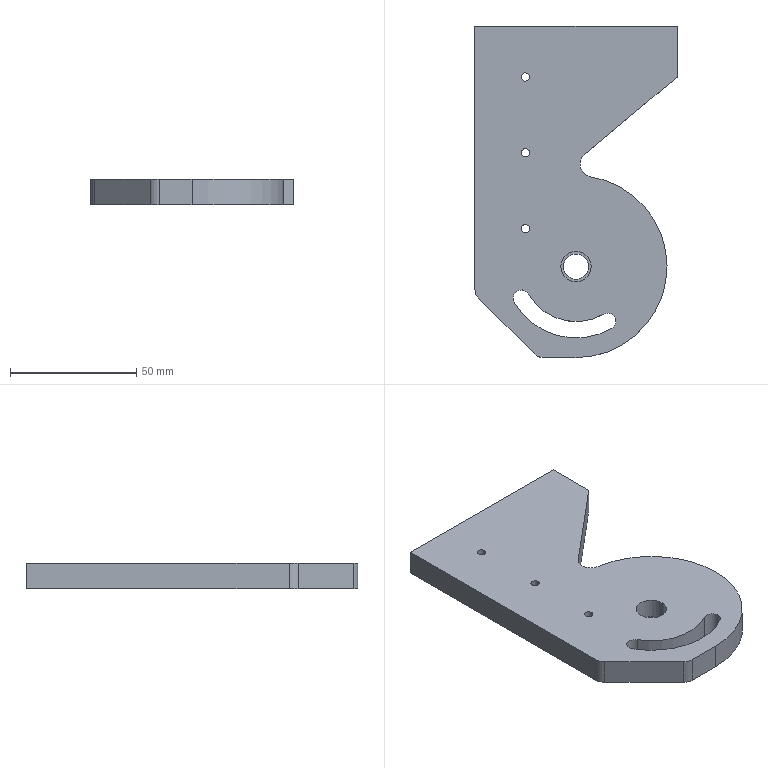Part | SolidWorks | features HoleWzd 3, Cut 1, Extrusion 1, Fillet 1, ICE 1 | 1 solid | 37 faces | box 80 x 131 x 10 mm | volume 79591 mm3 | cylinder 24 | plane 9 | cone 4 | commonest cylinder face diameters 3.3 x6 10 x6 5 x4 6.5 x3 12 x2 43.5 x1
STEP:
#1=CARTESIAN_POINT('',(-18.35,35.,5.));
#2=VERTEX_POINT('',#1);
#3=CARTESIAN_POINT('',(-21.65,35.,5.));
#4=VERTEX_POINT('',#3);
#5=CARTESIAN_POINT('',(-20.,35.,5.));
#6=DIRECTION('',(0.,0.,-1.));
#7=DIRECTION('',(-1.,0.,0.));
#8=AXIS2_PLACEMENT_3D('',#5,#6,#7);
#9=CIRCLE('',#8,1.65);
#10=EDGE_CURVE('',#2,#4,#9,.T.);
#11=ORIENTED_EDGE('',*,*,#10,.F.);
#12=CARTESIAN_POINT('',(-18.35,35.,-5.));
#13=VERTEX_POINT('',#12);
#14=CARTESIAN_POINT('',(-18.35,35.,-5.));
#15=DIRECTION('',(0.,0.,-1.));
#16=VECTOR('',#15,1000.);
#17=LINE('',#14,#16);
#18=EDGE_CURVE('',#2,#13,#17,.T.);
#19=ORIENTED_EDGE('',*,*,#18,.T.);
#20=CARTESIAN_POINT('',(-21.65,35.,-5.));
#21=VERTEX_POINT('',#20);
#22=CARTESIAN_POINT('',(-20.,35.,-5.));
#23=DIRECTION('',(0.,0.,-1.));
#24=DIRECTION('',(-1.,0.,0.));
#25=AXIS2_PLACEMENT_3D('',#22,#23,#24);
#26=CIRCLE('',#25,1.65);
#27=EDGE_CURVE('',#13,#21,#26,.T.);
#28=ORIENTED_EDGE('',*,*,#27,.T.);
#29=CARTESIAN_POINT('',(-21.65,35.,-5.));
#30=DIRECTION('',(0.,0.,-1.));
#31=VECTOR('',#30,1000.);
#32=LINE('',#29,#31);
#33=EDGE_CURVE('',#4,#21,#32,.T.);
#34=ORIENTED_EDGE('',*,*,#33,.F.);
#35=EDGE_LOOP('',(#11,#19,#28,#34));
#36=FACE_OUTER_BOUND('',#35,.T.);
#37=CARTESIAN_POINT('',(-20.,35.,-5.));
#38=DIRECTION('',(0.,0.,-1.));
#39=DIRECTION('',(-1.,0.,0.));
#40=AXIS2_PLACEMENT_3D('',#37,#38,#39);
#41=CYLINDRICAL_SURFACE('',#40,1.65);
#42=ADVANCED_FACE('',(#36),#41,.F.);
#43=CARTESIAN_POINT('',(-18.35,65.,5.));
#44=VERTEX_POINT('',#43);
#45=CARTESIAN_POINT('',(-21.65,65.,5.));
#46=VERTEX_POINT('',#45);
#47=CARTESIAN_POINT('',(-20.,65.,5.));
#48=DIRECTION('',(0.,0.,-1.));
#49=DIRECTION('',(-1.,0.,0.));
#50=AXIS2_PLACEMENT_3D('',#47,#48,#49);
#51=CIRCLE('',#50,1.65);
#52=EDGE_CURVE('',#44,#46,#51,.T.);
#53=ORIENTED_EDGE('',*,*,#52,.F.);
#54=CARTESIAN_POINT('',(-18.35,65.,-5.));
#55=VERTEX_POINT('',#54);
#56=CARTESIAN_POINT('',(-18.35,65.,-5.));
#57=DIRECTION('',(0.,0.,-1.));
#58=VECTOR('',#57,1000.);
#59=LINE('',#56,#58);
#60=EDGE_CURVE('',#44,#55,#59,.T.);
#61=ORIENTED_EDGE('',*,*,#60,.T.);
#62=CARTESIAN_POINT('',(-21.65,65.,-5.));
#63=VERTEX_POINT('',#62);
#64=CARTESIAN_POINT('',(-20.,65.,-5.));
#65=DIRECTION('',(0.,0.,-1.));
#66=DIRECTION('',(-1.,0.,0.));
#67=AXIS2_PLACEMENT_3D('',#64,#65,#66);
#68=CIRCLE('',#67,1.65);
#69=EDGE_CURVE('',#55,#63,#68,.T.);
#70=ORIENTED_EDGE('',*,*,#69,.T.);
#71=CARTESIAN_POINT('',(-21.65,65.,-5.));
#72=DIRECTION('',(0.,0.,-1.));
#73=VECTOR('',#72,1000.);
#74=LINE('',#71,#73);
#75=EDGE_CURVE('',#46,#63,#74,.T.);
#76=ORIENTED_EDGE('',*,*,#75,.F.);
#77=EDGE_LOOP('',(#53,#61,#70,#76));
#78=FACE_OUTER_BOUND('',#77,.T.);
#79=CARTESIAN_POINT('',(-20.,65.,-5.));
#80=DIRECTION('',(0.,0.,-1.));
#81=DIRECTION('',(-1.,0.,0.));
#82=AXIS2_PLACEMENT_3D('',#79,#80,#81);
#83=CYLINDRICAL_SURFACE('',#82,1.65);
#84=ADVANCED_FACE('',(#78),#83,.F.);
#85=CARTESIAN_POINT('',(-18.35,5.,5.));
#86=VERTEX_POINT('',#85);
#87=CARTESIAN_POINT('',(-21.65,5.,5.));
#88=VERTEX_POINT('',#87);
#89=CARTESIAN_POINT('',(-20.,5.,5.));
#90=DIRECTION('',(0.,0.,-1.));
#91=DIRECTION('',(-1.,0.,0.));
#92=AXIS2_PLACEMENT_3D('',#89,#90,#91);
#93=CIRCLE('',#92,1.65);
#94=EDGE_CURVE('',#86,#88,#93,.T.);
#95=ORIENTED_EDGE('',*,*,#94,.F.);
#96=CARTESIAN_POINT('',(-18.35,5.,-5.));
#97=VERTEX_POINT('',#96);
#98=CARTESIAN_POINT('',(-18.35,5.,-5.));
#99=DIRECTION('',(0.,0.,-1.));
#100=VECTOR('',#99,1000.);
#101=LINE('',#98,#100);
#102=EDGE_CURVE('',#86,#97,#101,.T.);
#103=ORIENTED_EDGE('',*,*,#102,.T.);
#104=CARTESIAN_POINT('',(-21.65,5.,-5.));
#105=VERTEX_POINT('',#104);
#106=CARTESIAN_POINT('',(-20.,5.,-5.));
#107=DIRECTION('',(0.,0.,-1.));
#108=DIRECTION('',(-1.,0.,0.));
#109=AXIS2_PLACEMENT_3D('',#106,#107,#108);
#110=CIRCLE('',#109,1.65);
#111=EDGE_CURVE('',#97,#105,#110,.T.);
#112=ORIENTED_EDGE('',*,*,#111,.T.);
#113=CARTESIAN_POINT('',(-21.65,5.,-5.));
#114=DIRECTION('',(0.,0.,-1.));
#115=VECTOR('',#114,1000.);
#116=LINE('',#113,#115);
#117=EDGE_CURVE('',#88,#105,#116,.T.);
#118=ORIENTED_EDGE('',*,*,#117,.F.);
#119=EDGE_LOOP('',(#95,#103,#112,#118));
#120=FACE_OUTER_BOUND('',#119,.T.);
#121=CARTESIAN_POINT('',(-20.,5.,-5.));
#122=DIRECTION('',(0.,0.,-1.));
#123=DIRECTION('',(-1.,0.,0.));
#124=AXIS2_PLACEMENT_3D('',#121,#122,#123);
#125=CYLINDRICAL_SURFACE('',#124,1.65);
#126=ADVANCED_FACE('',(#120),#125,.F.);
#127=CARTESIAN_POINT('',(-28.,68.,-2.5));
#128=VERTEX_POINT('',#127);
#129=CARTESIAN_POINT('',(-28.,68.,2.5));
#130=VERTEX_POINT('',#129);
#131=CARTESIAN_POINT('',(-28.,68.,0.));
#132=DIRECTION('',(0.,1.,0.));
#133=DIRECTION('',(0.,0.,1.));
#134=AXIS2_PLACEMENT_3D('',#131,#132,#133);
#135=CIRCLE('',#134,2.5);
#136=EDGE_CURVE('',#128,#130,#135,.T.);
#137=ORIENTED_EDGE('',*,*,#136,.F.);
#138=CARTESIAN_POINT('',(-28.,85.,-2.5));
#139=VERTEX_POINT('',#138);
#140=CARTESIAN_POINT('',(-28.,85.,-2.5));
#141=DIRECTION('',(0.,1.,0.));
#142=VECTOR('',#141,1000.);
#143=LINE('',#140,#142);
#144=EDGE_CURVE('',#128,#139,#143,.T.);
#145=ORIENTED_EDGE('',*,*,#144,.T.);
#146=CARTESIAN_POINT('',(-28.,85.,2.5));
#147=VERTEX_POINT('',#146);
#148=CARTESIAN_POINT('',(-28.,85.,0.));
#149=DIRECTION('',(0.,1.,0.));
#150=DIRECTION('',(0.,0.,1.));
#151=AXIS2_PLACEMENT_3D('',#148,#149,#150);
#152=CIRCLE('',#151,2.5);
#153=EDGE_CURVE('',#139,#147,#152,.T.);
#154=ORIENTED_EDGE('',*,*,#153,.T.);
#155=CARTESIAN_POINT('',(-28.,85.,2.5));
#156=DIRECTION('',(0.,1.,0.));
#157=VECTOR('',#156,1000.);
#158=LINE('',#155,#157);
#159=EDGE_CURVE('',#130,#147,#158,.T.);
#160=ORIENTED_EDGE('',*,*,#159,.F.);
#161=EDGE_LOOP('',(#137,#145,#154,#160));
#162=FACE_OUTER_BOUND('',#161,.T.);
#163=CARTESIAN_POINT('',(-28.,85.,0.));
#164=DIRECTION('',(0.,1.,0.));
#165=DIRECTION('',(0.,0.,1.));
#166=AXIS2_PLACEMENT_3D('',#163,#164,#165);
#167=CYLINDRICAL_SURFACE('',#166,2.5);
#168=ADVANCED_FACE('',(#162),#167,.F.);
#169=CARTESIAN_POINT('',(-28.,66.498,0.));
#170=VERTEX_POINT('',#169);
#171=CARTESIAN_POINT('',(-28.,68.,2.5));
#172=DIRECTION('',(0.,0.515,0.8572));
#173=VECTOR('',#172,1000.);
#174=LINE('',#171,#173);
#175=EDGE_CURVE('',#170,#130,#174,.T.);
#176=ORIENTED_EDGE('',*,*,#175,.F.);
#177=CARTESIAN_POINT('',(-28.,68.,-2.5));
#178=DIRECTION('',(0.,0.515,-0.8572));
#179=VECTOR('',#178,1000.);
#180=LINE('',#177,#179);
#181=EDGE_CURVE('',#170,#128,#180,.T.);
#182=ORIENTED_EDGE('',*,*,#181,.T.);
#183=ORIENTED_EDGE('',*,*,#136,.T.);
#184=EDGE_LOOP('',(#176,#182,#183));
#185=FACE_OUTER_BOUND('',#184,.T.);
#186=CARTESIAN_POINT('',(-28.,68.,0.));
#187=DIRECTION('',(0.,1.,0.));
#188=DIRECTION('',(0.,0.,1.));
#189=AXIS2_PLACEMENT_3D('',#186,#187,#188);
#190=CONICAL_SURFACE('',#189,2.5,1.03);
#191=ADVANCED_FACE('',(#185),#190,.F.);
#192=CARTESIAN_POINT('',(28.,68.,-2.5));
#193=VERTEX_POINT('',#192);
#194=CARTESIAN_POINT('',(28.,68.,2.5));
#195=VERTEX_POINT('',#194);
#196=CARTESIAN_POINT('',(28.,68.,0.));
#197=DIRECTION('',(0.,1.,0.));
#198=DIRECTION('',(0.,0.,1.));
#199=AXIS2_PLACEMENT_3D('',#196,#197,#198);
#200=CIRCLE('',#199,2.5);
#201=EDGE_CURVE('',#193,#195,#200,.T.);
#202=ORIENTED_EDGE('',*,*,#201,.F.);
#203=CARTESIAN_POINT('',(28.,85.,-2.5));
#204=VERTEX_POINT('',#203);
#205=CARTESIAN_POINT('',(28.,85.,-2.5));
#206=DIRECTION('',(0.,1.,0.));
#207=VECTOR('',#206,1000.);
#208=LINE('',#205,#207);
#209=EDGE_CURVE('',#193,#204,#208,.T.);
#210=ORIENTED_EDGE('',*,*,#209,.T.);
#211=CARTESIAN_POINT('',(28.,85.,2.5));
#212=VERTEX_POINT('',#211);
#213=CARTESIAN_POINT('',(28.,85.,0.));
#214=DIRECTION('',(0.,1.,0.));
#215=DIRECTION('',(0.,0.,1.));
#216=AXIS2_PLACEMENT_3D('',#213,#214,#215);
#217=CIRCLE('',#216,2.5);
#218=EDGE_CURVE('',#204,#212,#217,.T.);
#219=ORIENTED_EDGE('',*,*,#218,.T.);
#220=CARTESIAN_POINT('',(28.,85.,2.5));
#221=DIRECTION('',(0.,1.,0.));
#222=VECTOR('',#221,1000.);
#223=LINE('',#220,#222);
#224=EDGE_CURVE('',#195,#212,#223,.T.);
#225=ORIENTED_EDGE('',*,*,#224,.F.);
#226=EDGE_LOOP('',(#202,#210,#219,#225));
#227=FACE_OUTER_BOUND('',#226,.T.);
#228=CARTESIAN_POINT('',(28.,85.,0.));
#229=DIRECTION('',(0.,1.,0.));
#230=DIRECTION('',(0.,0.,1.));
#231=AXIS2_PLACEMENT_3D('',#228,#229,#230);
#232=CYLINDRICAL_SURFACE('',#231,2.5);
#233=ADVANCED_FACE('',(#227),#232,.F.);
#234=CARTESIAN_POINT('',(28.,66.498,0.));
#235=VERTEX_POINT('',#234);
#236=CARTESIAN_POINT('',(28.,68.,2.5));
#237=DIRECTION('',(0.,0.515,0.8572));
#238=VECTOR('',#237,1000.);
#239=LINE('',#236,#238);
#240=EDGE_CURVE('',#235,#195,#239,.T.);
#241=ORIENTED_EDGE('',*,*,#240,.F.);
#242=CARTESIAN_POINT('',(28.,68.,-2.5));
#243=DIRECTION('',(0.,0.515,-0.8572));
#244=VECTOR('',#243,1000.);
#245=LINE('',#242,#244);
#246=EDGE_CURVE('',#235,#193,#245,.T.);
#247=ORIENTED_EDGE('',*,*,#246,.T.);
#248=ORIENTED_EDGE('',*,*,#201,.T.);
#249=EDGE_LOOP('',(#241,#247,#248));
#250=FACE_OUTER_BOUND('',#249,.T.);
#251=CARTESIAN_POINT('',(28.,68.,0.));
#252=DIRECTION('',(0.,1.,0.));
#253=DIRECTION('',(0.,0.,1.));
#254=AXIS2_PLACEMENT_3D('',#251,#252,#253);
#255=CONICAL_SURFACE('',#254,2.5,1.03);
#256=ADVANCED_FACE('',(#250),#255,.F.);
#257=CARTESIAN_POINT('',(1.618,30.462,5.));
#258=VERTEX_POINT('',#257);
#259=CARTESIAN_POINT('',(3.404,34.293,5.));
#260=VERTEX_POINT('',#259);
#261=CARTESIAN_POINT('',(6.618,30.462,5.));
#262=DIRECTION('',(0.,0.,-1.));
#263=DIRECTION('',(-1.,0.,0.));
#264=AXIS2_PLACEMENT_3D('',#261,#262,#263);
#265=CIRCLE('',#264,5.);
#266=EDGE_CURVE('',#258,#260,#265,.T.);
#267=ORIENTED_EDGE('',*,*,#266,.F.);
#268=CARTESIAN_POINT('',(1.618,30.462,-5.));
#269=VERTEX_POINT('',#268);
#270=CARTESIAN_POINT('',(1.618,30.462,5.));
#271=DIRECTION('',(0.,0.,-1.));
#272=VECTOR('',#271,1000.);
#273=LINE('',#270,#272);
#274=EDGE_CURVE('',#258,#269,#273,.T.);
#275=ORIENTED_EDGE('',*,*,#274,.T.);
#276=CARTESIAN_POINT('',(3.404,34.293,-5.));
#277=VERTEX_POINT('',#276);
#278=CARTESIAN_POINT('',(6.618,30.462,-5.));
#279=DIRECTION('',(0.,0.,1.));
#280=DIRECTION('',(-1.,0.,0.));
#281=AXIS2_PLACEMENT_3D('',#278,#279,#280);
#282=CIRCLE('',#281,5.);
#283=EDGE_CURVE('',#277,#269,#282,.T.);
#284=ORIENTED_EDGE('',*,*,#283,.F.);
#285=CARTESIAN_POINT('',(3.404,34.293,-5.));
#286=DIRECTION('',(0.,0.,-1.));
#287=VECTOR('',#286,1000.);
#288=LINE('',#285,#287);
#289=EDGE_CURVE('',#260,#277,#288,.T.);
#290=ORIENTED_EDGE('',*,*,#289,.F.);
#291=EDGE_LOOP('',(#267,#275,#284,#290));
#292=FACE_OUTER_BOUND('',#291,.T.);
#293=CARTESIAN_POINT('',(6.618,30.462,5.));
#294=DIRECTION('',(0.,0.,-1.));
#295=DIRECTION('',(-1.,0.,0.));
#296=AXIS2_PLACEMENT_3D('',#293,#294,#295);
#297=CYLINDRICAL_SURFACE('',#296,5.);
#298=ADVANCED_FACE('',(#292),#297,.F.);
#299=CARTESIAN_POINT('',(-24.901,-22.5,5.));
#300=VERTEX_POINT('',#299);
#301=CARTESIAN_POINT('',(-18.836,-20.875,5.));
#302=VERTEX_POINT('',#301);
#303=CARTESIAN_POINT('',(-21.651,-22.5,5.));
#304=DIRECTION('',(0.,0.,-1.));
#305=DIRECTION('',(-1.,0.,0.));
#306=AXIS2_PLACEMENT_3D('',#303,#304,#305);
#307=CIRCLE('',#306,3.25);
#308=EDGE_CURVE('',#300,#302,#307,.T.);
#309=ORIENTED_EDGE('',*,*,#308,.F.);
#310=CARTESIAN_POINT('',(-24.901,-22.5,-5.));
#311=VERTEX_POINT('',#310);
#312=CARTESIAN_POINT('',(-24.901,-22.5,5.));
#313=DIRECTION('',(0.,0.,-1.));
#314=VECTOR('',#313,1000.);
#315=LINE('',#312,#314);
#316=EDGE_CURVE('',#300,#311,#315,.T.);
#317=ORIENTED_EDGE('',*,*,#316,.T.);
#318=CARTESIAN_POINT('',(-18.836,-20.875,-5.));
#319=VERTEX_POINT('',#318);
#320=CARTESIAN_POINT('',(-21.651,-22.5,-5.));
#321=DIRECTION('',(0.,0.,-1.));
#322=DIRECTION('',(-1.,0.,0.));
#323=AXIS2_PLACEMENT_3D('',#320,#321,#322);
#324=CIRCLE('',#323,3.25);
#325=EDGE_CURVE('',#311,#319,#324,.T.);
#326=ORIENTED_EDGE('',*,*,#325,.T.);
#327=CARTESIAN_POINT('',(-18.836,-20.875,5.));
#328=DIRECTION('',(0.,0.,-1.));
#329=VECTOR('',#328,1000.);
#330=LINE('',#327,#329);
#331=EDGE_CURVE('',#302,#319,#330,.T.);
#332=ORIENTED_EDGE('',*,*,#331,.F.);
#333=EDGE_LOOP('',(#309,#317,#326,#332));
#334=FACE_OUTER_BOUND('',#333,.T.);
#335=CARTESIAN_POINT('',(-21.651,-22.5,5.));
#336=DIRECTION('',(0.,0.,-1.));
#337=DIRECTION('',(-1.,0.,0.));
#338=AXIS2_PLACEMENT_3D('',#335,#336,#337);
#339=CYLINDRICAL_SURFACE('',#338,3.25);
#340=ADVANCED_FACE('',(#334),#339,.F.);
#341=CARTESIAN_POINT('',(-6.,-10.,-3.));
#342=VERTEX_POINT('',#341);
#343=CARTESIAN_POINT('',(6.,-10.,-3.));
#344=VERTEX_POINT('',#343);
#345=CARTESIAN_POINT('',(0.,-10.,-3.));
#346=DIRECTION('',(0.,0.,1.));
#347=DIRECTION('',(1.,0.,0.));
#348=AXIS2_PLACEMENT_3D('',#345,#346,#347);
#349=CIRCLE('',#348,6.);
#350=EDGE_CURVE('',#342,#344,#349,.T.);
#351=ORIENTED_EDGE('',*,*,#350,.F.);
#352=CARTESIAN_POINT('',(-6.,-10.,5.));
#353=VERTEX_POINT('',#352);
#354=CARTESIAN_POINT('',(-6.,-10.,5.));
#355=DIRECTION('',(0.,0.,1.));
#356=VECTOR('',#355,1000.);
#357=LINE('',#354,#356);
#358=EDGE_CURVE('',#342,#353,#357,.T.);
#359=ORIENTED_EDGE('',*,*,#358,.T.);
#360=CARTESIAN_POINT('',(6.,-10.,5.));
#361=VERTEX_POINT('',#360);
#362=CARTESIAN_POINT('',(0.,-10.,5.));
#363=DIRECTION('',(0.,0.,1.));
#364=DIRECTION('',(1.,0.,0.));
#365=AXIS2_PLACEMENT_3D('',#362,#363,#364);
#366=CIRCLE('',#365,6.);
#367=EDGE_CURVE('',#353,#361,#366,.T.);
#368=ORIENTED_EDGE('',*,*,#367,.T.);
#369=CARTESIAN_POINT('',(6.,-10.,5.));
#370=DIRECTION('',(0.,0.,1.));
#371=VECTOR('',#370,1000.);
#372=LINE('',#369,#371);
#373=EDGE_CURVE('',#344,#361,#372,.T.);
#374=ORIENTED_EDGE('',*,*,#373,.F.);
#375=EDGE_LOOP('',(#351,#359,#368,#374));
#376=FACE_OUTER_BOUND('',#375,.T.);
#377=CARTESIAN_POINT('',(0.,-10.,5.));
#378=DIRECTION('',(0.,0.,1.));
#379=DIRECTION('',(1.,0.,0.));
#380=AXIS2_PLACEMENT_3D('',#377,#378,#379);
#381=CYLINDRICAL_SURFACE('',#380,6.);
#382=ADVANCED_FACE('',(#376),#381,.F.);
#383=CARTESIAN_POINT('',(-5.,-10.,-5.));
#384=VERTEX_POINT('',#383);
#385=CARTESIAN_POINT('',(5.,-10.,-5.));
#386=VERTEX_POINT('',#385);
#387=CARTESIAN_POINT('',(0.,-10.,-5.));
#388=DIRECTION('',(0.,0.,1.));
#389=DIRECTION('',(1.,0.,0.));
#390=AXIS2_PLACEMENT_3D('',#387,#388,#389);
#391=CIRCLE('',#390,5.);
#392=EDGE_CURVE('',#384,#386,#391,.T.);
#393=ORIENTED_EDGE('',*,*,#392,.F.);
#394=CARTESIAN_POINT('',(-5.,-10.,-3.));
#395=VERTEX_POINT('',#394);
#396=CARTESIAN_POINT('',(-5.,-10.,5.));
#397=DIRECTION('',(0.,0.,1.));
#398=VECTOR('',#397,1000.);
#399=LINE('',#396,#398);
#400=EDGE_CURVE('',#384,#395,#399,.T.);
#401=ORIENTED_EDGE('',*,*,#400,.T.);
#402=CARTESIAN_POINT('',(5.,-10.,-3.));
#403=VERTEX_POINT('',#402);
#404=CARTESIAN_POINT('',(0.,-10.,-3.));
#405=DIRECTION('',(0.,0.,1.));
#406=DIRECTION('',(1.,0.,0.));
#407=AXIS2_PLACEMENT_3D('',#404,#405,#406);
#408=CIRCLE('',#407,5.);
#409=EDGE_CURVE('',#395,#403,#408,.T.);
#410=ORIENTED_EDGE('',*,*,#409,.T.);
#411=CARTESIAN_POINT('',(5.,-10.,5.));
#412=DIRECTION('',(0.,0.,1.));
#413=VECTOR('',#412,1000.);
#414=LINE('',#411,#413);
#415=EDGE_CURVE('',#386,#403,#414,.T.);
#416=ORIENTED_EDGE('',*,*,#415,.F.);
#417=EDGE_LOOP('',(#393,#401,#410,#416));
#418=FACE_OUTER_BOUND('',#417,.T.);
#419=CARTESIAN_POINT('',(0.,-10.,5.));
#420=DIRECTION('',(0.,0.,1.));
#421=DIRECTION('',(1.,0.,0.));
#422=AXIS2_PLACEMENT_3D('',#419,#420,#421);
#423=CYLINDRICAL_SURFACE('',#422,5.);
#424=ADVANCED_FACE('',(#418),#423,.F.);
#425=CARTESIAN_POINT('',(-20.,35.,5.));
#426=DIRECTION('',(0.,0.,-1.));
#427=DIRECTION('',(-1.,0.,0.));
#428=AXIS2_PLACEMENT_3D('',#425,#426,#427);
#429=CIRCLE('',#428,1.65);
#430=EDGE_CURVE('',#4,#2,#429,.T.);
#431=ORIENTED_EDGE('',*,*,#430,.T.);
#432=ORIENTED_EDGE('',*,*,#10,.T.);
#433=EDGE_LOOP('',(#431,#432));
#434=FACE_BOUND('',#433,.T.);
#435=CARTESIAN_POINT('',(-20.,65.,5.));
#436=DIRECTION('',(0.,0.,-1.));
#437=DIRECTION('',(-1.,0.,0.));
#438=AXIS2_PLACEMENT_3D('',#435,#436,#437);
#439=CIRCLE('',#438,1.65);
#440=EDGE_CURVE('',#46,#44,#439,.T.);
#441=ORIENTED_EDGE('',*,*,#440,.T.);
#442=ORIENTED_EDGE('',*,*,#52,.T.);
#443=EDGE_LOOP('',(#441,#442));
#444=FACE_BOUND('',#443,.T.);
#445=CARTESIAN_POINT('',(-20.,5.,5.));
#446=DIRECTION('',(0.,0.,-1.));
#447=DIRECTION('',(-1.,0.,0.));
#448=AXIS2_PLACEMENT_3D('',#445,#446,#447);
#449=CIRCLE('',#448,1.65);
#450=EDGE_CURVE('',#88,#86,#449,.T.);
#451=ORIENTED_EDGE('',*,*,#450,.T.);
#452=ORIENTED_EDGE('',*,*,#94,.T.);
#453=EDGE_LOOP('',(#451,#452));
#454=FACE_BOUND('',#453,.T.);
#455=CARTESIAN_POINT('',(0.,-10.,5.));
#456=DIRECTION('',(0.,0.,1.));
#457=DIRECTION('',(1.,0.,0.));
#458=AXIS2_PLACEMENT_3D('',#455,#456,#457);
#459=CIRCLE('',#458,6.);
#460=EDGE_CURVE('',#361,#353,#459,.T.);
#461=ORIENTED_EDGE('',*,*,#460,.F.);
#462=ORIENTED_EDGE('',*,*,#367,.F.);
#463=EDGE_LOOP('',(#461,#462));
#464=FACE_BOUND('',#463,.T.);
#465=CARTESIAN_POINT('',(-40.,85.,5.));
#466=VERTEX_POINT('',#465);
#467=CARTESIAN_POINT('',(-40.,-18.929,5.));
#468=VERTEX_POINT('',#467);
#469=CARTESIAN_POINT('',(-40.,-85.,5.));
#470=DIRECTION('',(0.,-1.,0.));
#471=VECTOR('',#470,1000.);
#472=LINE('',#469,#471);
#473=EDGE_CURVE('',#466,#468,#472,.T.);
#474=ORIENTED_EDGE('',*,*,#473,.T.);
#475=CARTESIAN_POINT('',(-38.536,-22.464,5.));
#476=VERTEX_POINT('',#475);
#477=CARTESIAN_POINT('',(-35.,-18.929,5.));
#478=DIRECTION('',(0.,0.,1.));
#479=DIRECTION('',(-1.,0.,0.));
#480=AXIS2_PLACEMENT_3D('',#477,#478,#479);
#481=CIRCLE('',#480,5.);
#482=EDGE_CURVE('',#468,#476,#481,.T.);
#483=ORIENTED_EDGE('',*,*,#482,.T.);
#484=CARTESIAN_POINT('',(-16.464,-44.536,5.));
#485=VERTEX_POINT('',#484);
#486=CARTESIAN_POINT('',(-15.,-46.,5.));
#487=DIRECTION('',(0.7071,-0.7071,0.));
#488=VECTOR('',#487,1000.);
#489=LINE('',#486,#488);
#490=EDGE_CURVE('',#476,#485,#489,.T.);
#491=ORIENTED_EDGE('',*,*,#490,.T.);
#492=CARTESIAN_POINT('',(-12.929,-46.,5.));
#493=VERTEX_POINT('',#492);
#494=CARTESIAN_POINT('',(-12.929,-41.,5.));
#495=DIRECTION('',(0.,0.,1.));
#496=DIRECTION('',(-1.,0.,0.));
#497=AXIS2_PLACEMENT_3D('',#494,#495,#496);
#498=CIRCLE('',#497,5.);
#499=EDGE_CURVE('',#485,#493,#498,.T.);
#500=ORIENTED_EDGE('',*,*,#499,.T.);
#501=CARTESIAN_POINT('',(0.,-46.,5.));
#502=VERTEX_POINT('',#501);
#503=CARTESIAN_POINT('',(0.,-46.,5.));
#504=DIRECTION('',(1.,0.,0.));
#505=VECTOR('',#504,1000.);
#506=LINE('',#503,#505);
#507=EDGE_CURVE('',#493,#502,#506,.T.);
#508=ORIENTED_EDGE('',*,*,#507,.T.);
#509=CARTESIAN_POINT('',(5.811,25.528,5.));
#510=VERTEX_POINT('',#509);
#511=CARTESIAN_POINT('',(0.,-10.,5.));
#512=DIRECTION('',(0.,0.,1.));
#513=DIRECTION('',(-1.,0.,0.));
#514=AXIS2_PLACEMENT_3D('',#511,#512,#513);
#515=CIRCLE('',#514,36.);
#516=EDGE_CURVE('',#502,#510,#515,.T.);
#517=ORIENTED_EDGE('',*,*,#516,.T.);
#518=CARTESIAN_POINT('',(6.618,30.462,5.));
#519=DIRECTION('',(0.,0.,-1.));
#520=DIRECTION('',(-1.,0.,0.));
#521=AXIS2_PLACEMENT_3D('',#518,#519,#520);
#522=CIRCLE('',#521,5.);
#523=EDGE_CURVE('',#510,#258,#522,.T.);
#524=ORIENTED_EDGE('',*,*,#523,.T.);
#525=ORIENTED_EDGE('',*,*,#266,.T.);
#526=CARTESIAN_POINT('',(40.,65.,5.));
#527=VERTEX_POINT('',#526);
#528=CARTESIAN_POINT('',(-7.393,25.233,5.));
#529=DIRECTION('',(0.766,0.6428,0.));
#530=VECTOR('',#529,1000.);
#531=LINE('',#528,#530);
#532=EDGE_CURVE('',#260,#527,#531,.T.);
#533=ORIENTED_EDGE('',*,*,#532,.T.);
#534=CARTESIAN_POINT('',(40.,85.,5.));
#535=VERTEX_POINT('',#534);
#536=CARTESIAN_POINT('',(40.,-85.,5.));
#537=DIRECTION('',(0.,1.,0.));
#538=VECTOR('',#537,1000.);
#539=LINE('',#536,#538);
#540=EDGE_CURVE('',#527,#535,#539,.T.);
#541=ORIENTED_EDGE('',*,*,#540,.T.);
#542=CARTESIAN_POINT('',(-40.,85.,5.));
#543=DIRECTION('',(-1.,0.,0.));
#544=VECTOR('',#543,1000.);
#545=LINE('',#542,#544);
#546=EDGE_CURVE('',#535,#466,#545,.T.);
#547=ORIENTED_EDGE('',*,*,#546,.T.);
#548=EDGE_LOOP('',(#474,#483,#491,#500,#508,#517,#524,#525,#533,#541,#547));
#549=FACE_OUTER_BOUND('',#548,.T.);
#550=CARTESIAN_POINT('',(14.125,-34.465,5.));
#551=VERTEX_POINT('',#550);
#552=CARTESIAN_POINT('',(-24.465,-24.125,5.));
#553=VERTEX_POINT('',#552);
#554=CARTESIAN_POINT('',(0.,-10.,5.));
#555=DIRECTION('',(0.,0.,-1.));
#556=DIRECTION('',(-1.,0.,0.));
#557=AXIS2_PLACEMENT_3D('',#554,#555,#556);
#558=CIRCLE('',#557,28.25);
#559=EDGE_CURVE('',#551,#553,#558,.T.);
#560=ORIENTED_EDGE('',*,*,#559,.T.);
#561=CARTESIAN_POINT('',(-21.651,-22.5,5.));
#562=DIRECTION('',(0.,0.,-1.));
#563=DIRECTION('',(-1.,0.,0.));
#564=AXIS2_PLACEMENT_3D('',#561,#562,#563);
#565=CIRCLE('',#564,3.25);
#566=EDGE_CURVE('',#553,#300,#565,.T.);
#567=ORIENTED_EDGE('',*,*,#566,.T.);
#568=ORIENTED_EDGE('',*,*,#308,.T.);
#569=CARTESIAN_POINT('',(10.875,-28.836,5.));
#570=VERTEX_POINT('',#569);
#571=CARTESIAN_POINT('',(0.,-10.,5.));
#572=DIRECTION('',(0.,0.,1.));
#573=DIRECTION('',(-1.,0.,0.));
#574=AXIS2_PLACEMENT_3D('',#571,#572,#573);
#575=CIRCLE('',#574,21.75);
#576=EDGE_CURVE('',#302,#570,#575,.T.);
#577=ORIENTED_EDGE('',*,*,#576,.T.);
#578=CARTESIAN_POINT('',(12.5,-31.651,5.));
#579=DIRECTION('',(0.,0.,-1.));
#580=DIRECTION('',(-1.,0.,0.));
#581=AXIS2_PLACEMENT_3D('',#578,#579,#580);
#582=CIRCLE('',#581,3.25);
#583=EDGE_CURVE('',#570,#551,#582,.T.);
#584=ORIENTED_EDGE('',*,*,#583,.T.);
#585=EDGE_LOOP('',(#560,#567,#568,#577,#584));
#586=FACE_BOUND('',#585,.T.);
#587=CARTESIAN_POINT('',(0.,0.,5.));
#588=DIRECTION('',(0.,0.,-1.));
#589=DIRECTION('',(-1.,0.,0.));
#590=AXIS2_PLACEMENT_3D('',#587,#588,#589);
#591=PLANE('',#590);
#592=ADVANCED_FACE('',(#434,#444,#454,#464,#549,#586),#591,.F.);
#593=CARTESIAN_POINT('',(-20.,35.,-5.));
#594=DIRECTION('',(0.,0.,-1.));
#595=DIRECTION('',(-1.,0.,0.));
#596=AXIS2_PLACEMENT_3D('',#593,#594,#595);
#597=CIRCLE('',#596,1.65);
#598=EDGE_CURVE('',#21,#13,#597,.T.);
#599=ORIENTED_EDGE('',*,*,#598,.F.);
#600=ORIENTED_EDGE('',*,*,#27,.F.);
#601=EDGE_LOOP('',(#599,#600));
#602=FACE_BOUND('',#601,.T.);
#603=CARTESIAN_POINT('',(-20.,65.,-5.));
#604=DIRECTION('',(0.,0.,-1.));
#605=DIRECTION('',(-1.,0.,0.));
#606=AXIS2_PLACEMENT_3D('',#603,#604,#605);
#607=CIRCLE('',#606,1.65);
#608=EDGE_CURVE('',#63,#55,#607,.T.);
#609=ORIENTED_EDGE('',*,*,#608,.F.);
#610=ORIENTED_EDGE('',*,*,#69,.F.);
#611=EDGE_LOOP('',(#609,#610));
#612=FACE_BOUND('',#611,.T.);
#613=CARTESIAN_POINT('',(-20.,5.,-5.));
#614=DIRECTION('',(0.,0.,-1.));
#615=DIRECTION('',(-1.,0.,0.));
#616=AXIS2_PLACEMENT_3D('',#613,#614,#615);
#617=CIRCLE('',#616,1.65);
#618=EDGE_CURVE('',#105,#97,#617,.T.);
#619=ORIENTED_EDGE('',*,*,#618,.F.);
#620=ORIENTED_EDGE('',*,*,#111,.F.);
#621=EDGE_LOOP('',(#619,#620));
#622=FACE_BOUND('',#621,.T.);
#623=CARTESIAN_POINT('',(-38.536,-22.464,-5.));
#624=VERTEX_POINT('',#623);
#625=CARTESIAN_POINT('',(-16.464,-44.536,-5.));
#626=VERTEX_POINT('',#625);
#627=CARTESIAN_POINT('',(-15.,-46.,-5.));
#628=DIRECTION('',(0.7071,-0.7071,0.));
#629=VECTOR('',#628,1000.);
#630=LINE('',#627,#629);
#631=EDGE_CURVE('',#624,#626,#630,.T.);
#632=ORIENTED_EDGE('',*,*,#631,.F.);
#633=CARTESIAN_POINT('',(-40.,-18.929,-5.));
#634=VERTEX_POINT('',#633);
#635=CARTESIAN_POINT('',(-35.,-18.929,-5.));
#636=DIRECTION('',(0.,0.,-1.));
#637=DIRECTION('',(-1.,0.,0.));
#638=AXIS2_PLACEMENT_3D('',#635,#636,#637);
#639=CIRCLE('',#638,5.);
#640=EDGE_CURVE('',#624,#634,#639,.T.);
#641=ORIENTED_EDGE('',*,*,#640,.T.);
#642=CARTESIAN_POINT('',(-40.,85.,-5.));
#643=VERTEX_POINT('',#642);
#644=CARTESIAN_POINT('',(-40.,-85.,-5.));
#645=DIRECTION('',(0.,-1.,0.));
#646=VECTOR('',#645,1000.);
#647=LINE('',#644,#646);
#648=EDGE_CURVE('',#643,#634,#647,.T.);
#649=ORIENTED_EDGE('',*,*,#648,.F.);
#650=CARTESIAN_POINT('',(40.,85.,-5.));
#651=VERTEX_POINT('',#650);
#652=CARTESIAN_POINT('',(-40.,85.,-5.));
#653=DIRECTION('',(-1.,0.,0.));
#654=VECTOR('',#653,1000.);
#655=LINE('',#652,#654);
#656=EDGE_CURVE('',#651,#643,#655,.T.);
#657=ORIENTED_EDGE('',*,*,#656,.F.);
#658=CARTESIAN_POINT('',(40.,65.,-5.));
#659=VERTEX_POINT('',#658);
#660=CARTESIAN_POINT('',(40.,-85.,-5.));
#661=DIRECTION('',(0.,1.,0.));
#662=VECTOR('',#661,1000.);
#663=LINE('',#660,#662);
#664=EDGE_CURVE('',#659,#651,#663,.T.);
#665=ORIENTED_EDGE('',*,*,#664,.F.);
#666=CARTESIAN_POINT('',(-7.393,25.233,-5.));
#667=DIRECTION('',(0.766,0.6428,0.));
#668=VECTOR('',#667,1000.);
#669=LINE('',#666,#668);
#670=EDGE_CURVE('',#277,#659,#669,.T.);
#671=ORIENTED_EDGE('',*,*,#670,.F.);
#672=ORIENTED_EDGE('',*,*,#283,.T.);
#673=CARTESIAN_POINT('',(5.811,25.528,-5.));
#674=VERTEX_POINT('',#673);
#675=CARTESIAN_POINT('',(6.618,30.462,-5.));
#676=DIRECTION('',(0.,0.,1.));
#677=DIRECTION('',(-1.,0.,0.));
#678=AXIS2_PLACEMENT_3D('',#675,#676,#677);
#679=CIRCLE('',#678,5.);
#680=EDGE_CURVE('',#269,#674,#679,.T.);
#681=ORIENTED_EDGE('',*,*,#680,.T.);
#682=CARTESIAN_POINT('',(0.,-46.,-5.));
#683=VERTEX_POINT('',#682);
#684=CARTESIAN_POINT('',(0.,-10.,-5.));
#685=DIRECTION('',(0.,0.,1.));
#686=DIRECTION('',(-1.,0.,0.));
#687=AXIS2_PLACEMENT_3D('',#684,#685,#686);
#688=CIRCLE('',#687,36.);
#689=EDGE_CURVE('',#683,#674,#688,.T.);
#690=ORIENTED_EDGE('',*,*,#689,.F.);
#691=CARTESIAN_POINT('',(-12.929,-46.,-5.));
#692=VERTEX_POINT('',#691);
#693=CARTESIAN_POINT('',(0.,-46.,-5.));
#694=DIRECTION('',(1.,0.,0.));
#695=VECTOR('',#694,1000.);
#696=LINE('',#693,#695);
#697=EDGE_CURVE('',#692,#683,#696,.T.);
#698=ORIENTED_EDGE('',*,*,#697,.F.);
#699=CARTESIAN_POINT('',(-12.929,-41.,-5.));
#700=DIRECTION('',(0.,0.,-1.));
#701=DIRECTION('',(-1.,0.,0.));
#702=AXIS2_PLACEMENT_3D('',#699,#700,#701);
#703=CIRCLE('',#702,5.);
#704=EDGE_CURVE('',#692,#626,#703,.T.);
#705=ORIENTED_EDGE('',*,*,#704,.T.);
#706=EDGE_LOOP('',(#632,#641,#649,#657,#665,#671,#672,#681,#690,#698,#705));
#707=FACE_OUTER_BOUND('',#706,.T.);
#708=CARTESIAN_POINT('',(0.,-10.,-5.));
#709=DIRECTION('',(0.,0.,1.));
#710=DIRECTION('',(1.,0.,0.));
#711=AXIS2_PLACEMENT_3D('',#708,#709,#710);
#712=CIRCLE('',#711,5.);
#713=EDGE_CURVE('',#386,#384,#712,.T.);
#714=ORIENTED_EDGE('',*,*,#713,.T.);
#715=ORIENTED_EDGE('',*,*,#392,.T.);
#716=EDGE_LOOP('',(#714,#715));
#717=FACE_BOUND('',#716,.T.);
#718=CARTESIAN_POINT('',(-24.465,-24.125,-5.));
#719=VERTEX_POINT('',#718);
#720=CARTESIAN_POINT('',(-21.651,-22.5,-5.));
#721=DIRECTION('',(0.,0.,-1.));
#722=DIRECTION('',(-1.,0.,0.));
#723=AXIS2_PLACEMENT_3D('',#720,#721,#722);
#724=CIRCLE('',#723,3.25);
#725=EDGE_CURVE('',#719,#311,#724,.T.);
#726=ORIENTED_EDGE('',*,*,#725,.F.);
#727=CARTESIAN_POINT('',(14.125,-34.465,-5.));
#728=VERTEX_POINT('',#727);
#729=CARTESIAN_POINT('',(0.,-10.,-5.));
#730=DIRECTION('',(0.,0.,-1.));
#731=DIRECTION('',(-1.,0.,0.));
#732=AXIS2_PLACEMENT_3D('',#729,#730,#731);
#733=CIRCLE('',#732,28.25);
#734=EDGE_CURVE('',#728,#719,#733,.T.);
#735=ORIENTED_EDGE('',*,*,#734,.F.);
#736=CARTESIAN_POINT('',(10.875,-28.836,-5.));
#737=VERTEX_POINT('',#736);
#738=CARTESIAN_POINT('',(12.5,-31.651,-5.));
#739=DIRECTION('',(0.,0.,-1.));
#740=DIRECTION('',(-1.,0.,0.));
#741=AXIS2_PLACEMENT_3D('',#738,#739,#740);
#742=CIRCLE('',#741,3.25);
#743=EDGE_CURVE('',#737,#728,#742,.T.);
#744=ORIENTED_EDGE('',*,*,#743,.F.);
#745=CARTESIAN_POINT('',(0.,-10.,-5.));
#746=DIRECTION('',(0.,0.,1.));
#747=DIRECTION('',(-1.,0.,0.));
#748=AXIS2_PLACEMENT_3D('',#745,#746,#747);
#749=CIRCLE('',#748,21.75);
#750=EDGE_CURVE('',#319,#737,#749,.T.);
#751=ORIENTED_EDGE('',*,*,#750,.F.);
#752=ORIENTED_EDGE('',*,*,#325,.F.);
#753=EDGE_LOOP('',(#726,#735,#744,#751,#752));
#754=FACE_BOUND('',#753,.T.);
#755=CARTESIAN_POINT('',(0.,0.,-5.));
#756=DIRECTION('',(0.,0.,-1.));
#757=DIRECTION('',(-1.,0.,0.));
#758=AXIS2_PLACEMENT_3D('',#755,#756,#757);
#759=PLANE('',#758);
#760=ADVANCED_FACE('',(#602,#612,#622,#707,#717,#754),#759,.T.);
#761=ORIENTED_EDGE('',*,*,#540,.F.);
#762=CARTESIAN_POINT('',(40.,65.,5.));
#763=DIRECTION('',(0.,0.,-1.));
#764=VECTOR('',#763,1000.);
#765=LINE('',#762,#764);
#766=EDGE_CURVE('',#527,#659,#765,.T.);
#767=ORIENTED_EDGE('',*,*,#766,.T.);
#768=ORIENTED_EDGE('',*,*,#664,.T.);
#769=CARTESIAN_POINT('',(40.,85.,5.));
#770=DIRECTION('',(0.,0.,-1.));
#771=VECTOR('',#770,1000.);
#772=LINE('',#769,#771);
#773=EDGE_CURVE('',#535,#651,#772,.T.);
#774=ORIENTED_EDGE('',*,*,#773,.F.);
#775=EDGE_LOOP('',(#761,#767,#768,#774));
#776=FACE_OUTER_BOUND('',#775,.T.);
#777=CARTESIAN_POINT('',(40.,-85.,5.));
#778=DIRECTION('',(-1.,0.,0.));
#779=DIRECTION('',(0.,0.,1.));
#780=AXIS2_PLACEMENT_3D('',#777,#778,#779);
#781=PLANE('',#780);
#782=ADVANCED_FACE('',(#776),#781,.F.);
#783=CARTESIAN_POINT('',(-28.,85.,0.));
#784=DIRECTION('',(0.,1.,0.));
#785=DIRECTION('',(0.,0.,1.));
#786=AXIS2_PLACEMENT_3D('',#783,#784,#785);
#787=CIRCLE('',#786,2.5);
#788=EDGE_CURVE('',#147,#139,#787,.T.);
#789=ORIENTED_EDGE('',*,*,#788,.F.);
#790=ORIENTED_EDGE('',*,*,#153,.F.);
#791=EDGE_LOOP('',(#789,#790));
#792=FACE_BOUND('',#791,.T.);
#793=CARTESIAN_POINT('',(28.,85.,0.));
#794=DIRECTION('',(0.,1.,0.));
#795=DIRECTION('',(0.,0.,1.));
#796=AXIS2_PLACEMENT_3D('',#793,#794,#795);
#797=CIRCLE('',#796,2.5);
#798=EDGE_CURVE('',#212,#204,#797,.T.);
#799=ORIENTED_EDGE('',*,*,#798,.F.);
#800=ORIENTED_EDGE('',*,*,#218,.F.);
#801=EDGE_LOOP('',(#799,#800));
#802=FACE_BOUND('',#801,.T.);
#803=ORIENTED_EDGE('',*,*,#656,.T.);
#804=CARTESIAN_POINT('',(-40.,85.,5.));
#805=DIRECTION('',(0.,0.,-1.));
#806=VECTOR('',#805,1000.);
#807=LINE('',#804,#806);
#808=EDGE_CURVE('',#466,#643,#807,.T.);
#809=ORIENTED_EDGE('',*,*,#808,.F.);
#810=ORIENTED_EDGE('',*,*,#546,.F.);
#811=ORIENTED_EDGE('',*,*,#773,.T.);
#812=EDGE_LOOP('',(#803,#809,#810,#811));
#813=FACE_OUTER_BOUND('',#812,.T.);
#814=CARTESIAN_POINT('',(-40.,85.,5.));
#815=DIRECTION('',(0.,-1.,0.));
#816=DIRECTION('',(0.,0.,-1.));
#817=AXIS2_PLACEMENT_3D('',#814,#815,#816);
#818=PLANE('',#817);
#819=ADVANCED_FACE('',(#792,#802,#813),#818,.F.);
#820=ORIENTED_EDGE('',*,*,#648,.T.);
#821=CARTESIAN_POINT('',(-40.,-18.929,5.));
#822=DIRECTION('',(0.,0.,1.));
#823=VECTOR('',#822,1000.);
#824=LINE('',#821,#823);
#825=EDGE_CURVE('',#634,#468,#824,.T.);
#826=ORIENTED_EDGE('',*,*,#825,.T.);
#827=ORIENTED_EDGE('',*,*,#473,.F.);
#828=ORIENTED_EDGE('',*,*,#808,.T.);
#829=EDGE_LOOP('',(#820,#826,#827,#828));
#830=FACE_OUTER_BOUND('',#829,.T.);
#831=CARTESIAN_POINT('',(-40.,-85.,5.));
#832=DIRECTION('',(1.,0.,0.));
#833=DIRECTION('',(0.,0.,-1.));
#834=AXIS2_PLACEMENT_3D('',#831,#832,#833);
#835=PLANE('',#834);
#836=ADVANCED_FACE('',(#830),#835,.F.);
#837=ORIENTED_EDGE('',*,*,#400,.F.);
#838=ORIENTED_EDGE('',*,*,#713,.F.);
#839=ORIENTED_EDGE('',*,*,#415,.T.);
#840=CARTESIAN_POINT('',(0.,-10.,-3.));
#841=DIRECTION('',(0.,0.,1.));
#842=DIRECTION('',(1.,0.,0.));
#843=AXIS2_PLACEMENT_3D('',#840,#841,#842);
#844=CIRCLE('',#843,5.);
#845=EDGE_CURVE('',#403,#395,#844,.T.);
#846=ORIENTED_EDGE('',*,*,#845,.T.);
#847=EDGE_LOOP('',(#837,#838,#839,#846));
#848=FACE_OUTER_BOUND('',#847,.T.);
#849=CARTESIAN_POINT('',(0.,-10.,5.));
#850=DIRECTION('',(0.,0.,1.));
#851=DIRECTION('',(1.,0.,0.));
#852=AXIS2_PLACEMENT_3D('',#849,#850,#851);
#853=CYLINDRICAL_SURFACE('',#852,5.);
#854=ADVANCED_FACE('',(#848),#853,.F.);
#855=ORIENTED_EDGE('',*,*,#845,.F.);
#856=ORIENTED_EDGE('',*,*,#409,.F.);
#857=EDGE_LOOP('',(#855,#856));
#858=FACE_BOUND('',#857,.T.);
#859=CARTESIAN_POINT('',(0.,-10.,-3.));
#860=DIRECTION('',(0.,0.,1.));
#861=DIRECTION('',(1.,0.,0.));
#862=AXIS2_PLACEMENT_3D('',#859,#860,#861);
#863=CIRCLE('',#862,6.);
#864=EDGE_CURVE('',#344,#342,#863,.T.);
#865=ORIENTED_EDGE('',*,*,#864,.T.);
#866=ORIENTED_EDGE('',*,*,#350,.T.);
#867=EDGE_LOOP('',(#865,#866));
#868=FACE_OUTER_BOUND('',#867,.T.);
#869=CARTESIAN_POINT('',(5.,-10.,-3.));
#870=DIRECTION('',(0.,0.,-1.));
#871=DIRECTION('',(-1.,0.,0.));
#872=AXIS2_PLACEMENT_3D('',#869,#870,#871);
#873=PLANE('',#872);
#874=ADVANCED_FACE('',(#858,#868),#873,.F.);
#875=ORIENTED_EDGE('',*,*,#358,.F.);
#876=ORIENTED_EDGE('',*,*,#864,.F.);
#877=ORIENTED_EDGE('',*,*,#373,.T.);
#878=ORIENTED_EDGE('',*,*,#460,.T.);
#879=EDGE_LOOP('',(#875,#876,#877,#878));
#880=FACE_OUTER_BOUND('',#879,.T.);
#881=CARTESIAN_POINT('',(0.,-10.,5.));
#882=DIRECTION('',(0.,0.,1.));
#883=DIRECTION('',(1.,0.,0.));
#884=AXIS2_PLACEMENT_3D('',#881,#882,#883);
#885=CYLINDRICAL_SURFACE('',#884,6.);
#886=ADVANCED_FACE('',(#880),#885,.F.);
#887=ORIENTED_EDGE('',*,*,#316,.F.);
#888=ORIENTED_EDGE('',*,*,#566,.F.);
#889=CARTESIAN_POINT('',(-24.465,-24.125,5.));
#890=DIRECTION('',(0.,0.,-1.));
#891=VECTOR('',#890,1000.);
#892=LINE('',#889,#891);
#893=EDGE_CURVE('',#553,#719,#892,.T.);
#894=ORIENTED_EDGE('',*,*,#893,.T.);
#895=ORIENTED_EDGE('',*,*,#725,.T.);
#896=EDGE_LOOP('',(#887,#888,#894,#895));
#897=FACE_OUTER_BOUND('',#896,.T.);
#898=CARTESIAN_POINT('',(-21.651,-22.5,5.));
#899=DIRECTION('',(0.,0.,-1.));
#900=DIRECTION('',(-1.,0.,0.));
#901=AXIS2_PLACEMENT_3D('',#898,#899,#900);
#902=CYLINDRICAL_SURFACE('',#901,3.25);
#903=ADVANCED_FACE('',(#897),#902,.F.);
#904=ORIENTED_EDGE('',*,*,#734,.T.);
#905=ORIENTED_EDGE('',*,*,#893,.F.);
#906=ORIENTED_EDGE('',*,*,#559,.F.);
#907=CARTESIAN_POINT('',(14.125,-34.465,5.));
#908=DIRECTION('',(0.,0.,-1.));
#909=VECTOR('',#908,1000.);
#910=LINE('',#907,#909);
#911=EDGE_CURVE('',#551,#728,#910,.T.);
#912=ORIENTED_EDGE('',*,*,#911,.T.);
#913=EDGE_LOOP('',(#904,#905,#906,#912));
#914=FACE_OUTER_BOUND('',#913,.T.);
#915=CARTESIAN_POINT('',(0.,-10.,5.));
#916=DIRECTION('',(0.,0.,-1.));
#917=DIRECTION('',(-1.,0.,0.));
#918=AXIS2_PLACEMENT_3D('',#915,#916,#917);
#919=CYLINDRICAL_SURFACE('',#918,28.25);
#920=ADVANCED_FACE('',(#914),#919,.F.);
#921=ORIENTED_EDGE('',*,*,#743,.T.);
#922=ORIENTED_EDGE('',*,*,#911,.F.);
#923=ORIENTED_EDGE('',*,*,#583,.F.);
#924=CARTESIAN_POINT('',(10.875,-28.836,5.));
#925=DIRECTION('',(0.,0.,-1.));
#926=VECTOR('',#925,1000.);
#927=LINE('',#924,#926);
#928=EDGE_CURVE('',#570,#737,#927,.T.);
#929=ORIENTED_EDGE('',*,*,#928,.T.);
#930=EDGE_LOOP('',(#921,#922,#923,#929));
#931=FACE_OUTER_BOUND('',#930,.T.);
#932=CARTESIAN_POINT('',(12.5,-31.651,5.));
#933=DIRECTION('',(0.,0.,-1.));
#934=DIRECTION('',(-1.,0.,0.));
#935=AXIS2_PLACEMENT_3D('',#932,#933,#934);
#936=CYLINDRICAL_SURFACE('',#935,3.25);
#937=ADVANCED_FACE('',(#931),#936,.F.);
#938=ORIENTED_EDGE('',*,*,#750,.T.);
#939=ORIENTED_EDGE('',*,*,#928,.F.);
#940=ORIENTED_EDGE('',*,*,#576,.F.);
#941=ORIENTED_EDGE('',*,*,#331,.T.);
#942=EDGE_LOOP('',(#938,#939,#940,#941));
#943=FACE_OUTER_BOUND('',#942,.T.);
#944=CARTESIAN_POINT('',(0.,-10.,5.));
#945=DIRECTION('',(0.,0.,-1.));
#946=DIRECTION('',(-1.,0.,0.));
#947=AXIS2_PLACEMENT_3D('',#944,#945,#946);
#948=CYLINDRICAL_SURFACE('',#947,21.75);
#949=ADVANCED_FACE('',(#943),#948,.T.);
#950=ORIENTED_EDGE('',*,*,#532,.F.);
#951=ORIENTED_EDGE('',*,*,#289,.T.);
#952=ORIENTED_EDGE('',*,*,#670,.T.);
#953=ORIENTED_EDGE('',*,*,#766,.F.);
#954=EDGE_LOOP('',(#950,#951,#952,#953));
#955=FACE_OUTER_BOUND('',#954,.T.);
#956=CARTESIAN_POINT('',(-7.393,25.233,5.));
#957=DIRECTION('',(-0.6428,0.766,0.));
#958=DIRECTION('',(-0.766,-0.6428,0.));
#959=AXIS2_PLACEMENT_3D('',#956,#957,#958);
#960=PLANE('',#959);
#961=ADVANCED_FACE('',(#955),#960,.F.);
#962=ORIENTED_EDGE('',*,*,#689,.T.);
#963=CARTESIAN_POINT('',(5.811,25.528,5.));
#964=DIRECTION('',(0.,0.,1.));
#965=VECTOR('',#964,1000.);
#966=LINE('',#963,#965);
#967=EDGE_CURVE('',#674,#510,#966,.T.);
#968=ORIENTED_EDGE('',*,*,#967,.T.);
#969=ORIENTED_EDGE('',*,*,#516,.F.);
#970=CARTESIAN_POINT('',(0.,-46.,5.));
#971=DIRECTION('',(0.,0.,-1.));
#972=VECTOR('',#971,1000.);
#973=LINE('',#970,#972);
#974=EDGE_CURVE('',#502,#683,#973,.T.);
#975=ORIENTED_EDGE('',*,*,#974,.T.);
#976=EDGE_LOOP('',(#962,#968,#969,#975));
#977=FACE_OUTER_BOUND('',#976,.T.);
#978=CARTESIAN_POINT('',(0.,-10.,5.));
#979=DIRECTION('',(0.,0.,-1.));
#980=DIRECTION('',(-1.,0.,0.));
#981=AXIS2_PLACEMENT_3D('',#978,#979,#980);
#982=CYLINDRICAL_SURFACE('',#981,36.);
#983=ADVANCED_FACE('',(#977),#982,.T.);
#984=ORIENTED_EDGE('',*,*,#507,.F.);
#985=CARTESIAN_POINT('',(-12.929,-46.,5.));
#986=DIRECTION('',(0.,0.,-1.));
#987=VECTOR('',#986,1000.);
#988=LINE('',#985,#987);
#989=EDGE_CURVE('',#493,#692,#988,.T.);
#990=ORIENTED_EDGE('',*,*,#989,.T.);
#991=ORIENTED_EDGE('',*,*,#697,.T.);
#992=ORIENTED_EDGE('',*,*,#974,.F.);
#993=EDGE_LOOP('',(#984,#990,#991,#992));
#994=FACE_OUTER_BOUND('',#993,.T.);
#995=CARTESIAN_POINT('',(0.,-46.,5.));
#996=DIRECTION('',(0.,1.,0.));
#997=DIRECTION('',(0.,0.,1.));
#998=AXIS2_PLACEMENT_3D('',#995,#996,#997);
#999=PLANE('',#998);
#1000=ADVANCED_FACE('',(#994),#999,.F.);
#1001=ORIENTED_EDGE('',*,*,#490,.F.);
#1002=CARTESIAN_POINT('',(-38.536,-22.464,5.));
#1003=DIRECTION('',(0.,0.,-1.));
#1004=VECTOR('',#1003,1000.);
#1005=LINE('',#1002,#1004);
#1006=EDGE_CURVE('',#476,#624,#1005,.T.);
#1007=ORIENTED_EDGE('',*,*,#1006,.T.);
#1008=ORIENTED_EDGE('',*,*,#631,.T.);
#1009=CARTESIAN_POINT('',(-16.464,-44.536,5.));
#1010=DIRECTION('',(0.,0.,1.));
#1011=VECTOR('',#1010,1000.);
#1012=LINE('',#1009,#1011);
#1013=EDGE_CURVE('',#626,#485,#1012,.T.);
#1014=ORIENTED_EDGE('',*,*,#1013,.T.);
#1015=EDGE_LOOP('',(#1001,#1007,#1008,#1014));
#1016=FACE_OUTER_BOUND('',#1015,.T.);
#1017=CARTESIAN_POINT('',(-15.,-46.,5.));
#1018=DIRECTION('',(0.7071,0.7071,0.));
#1019=DIRECTION('',(-0.7071,0.7071,0.));
#1020=AXIS2_PLACEMENT_3D('',#1017,#1018,#1019);
#1021=PLANE('',#1020);
#1022=ADVANCED_FACE('',(#1016),#1021,.F.);
#1023=ORIENTED_EDGE('',*,*,#482,.F.);
#1024=ORIENTED_EDGE('',*,*,#825,.F.);
#1025=ORIENTED_EDGE('',*,*,#640,.F.);
#1026=ORIENTED_EDGE('',*,*,#1006,.F.);
#1027=EDGE_LOOP('',(#1023,#1024,#1025,#1026));
#1028=FACE_OUTER_BOUND('',#1027,.T.);
#1029=CARTESIAN_POINT('',(-35.,-18.929,5.));
#1030=DIRECTION('',(0.,0.,-1.));
#1031=DIRECTION('',(-1.,0.,0.));
#1032=AXIS2_PLACEMENT_3D('',#1029,#1030,#1031);
#1033=CYLINDRICAL_SURFACE('',#1032,5.);
#1034=ADVANCED_FACE('',(#1028),#1033,.T.);
#1035=ORIENTED_EDGE('',*,*,#499,.F.);
#1036=ORIENTED_EDGE('',*,*,#1013,.F.);
#1037=ORIENTED_EDGE('',*,*,#704,.F.);
#1038=ORIENTED_EDGE('',*,*,#989,.F.);
#1039=EDGE_LOOP('',(#1035,#1036,#1037,#1038));
#1040=FACE_OUTER_BOUND('',#1039,.T.);
#1041=CARTESIAN_POINT('',(-12.929,-41.,5.));
#1042=DIRECTION('',(0.,0.,-1.));
#1043=DIRECTION('',(-1.,0.,0.));
#1044=AXIS2_PLACEMENT_3D('',#1041,#1042,#1043);
#1045=CYLINDRICAL_SURFACE('',#1044,5.);
#1046=ADVANCED_FACE('',(#1040),#1045,.T.);
#1047=ORIENTED_EDGE('',*,*,#274,.F.);
#1048=ORIENTED_EDGE('',*,*,#523,.F.);
#1049=ORIENTED_EDGE('',*,*,#967,.F.);
#1050=ORIENTED_EDGE('',*,*,#680,.F.);
#1051=EDGE_LOOP('',(#1047,#1048,#1049,#1050));
#1052=FACE_OUTER_BOUND('',#1051,.T.);
#1053=CARTESIAN_POINT('',(6.618,30.462,5.));
#1054=DIRECTION('',(0.,0.,-1.));
#1055=DIRECTION('',(-1.,0.,0.));
#1056=AXIS2_PLACEMENT_3D('',#1053,#1054,#1055);
#1057=CYLINDRICAL_SURFACE('',#1056,5.);
#1058=ADVANCED_FACE('',(#1052),#1057,.F.);
#1059=ORIENTED_EDGE('',*,*,#246,.F.);
#1060=ORIENTED_EDGE('',*,*,#240,.T.);
#1061=CARTESIAN_POINT('',(28.,68.,0.));
#1062=DIRECTION('',(0.,1.,0.));
#1063=DIRECTION('',(0.,0.,1.));
#1064=AXIS2_PLACEMENT_3D('',#1061,#1062,#1063);
#1065=CIRCLE('',#1064,2.5);
#1066=EDGE_CURVE('',#195,#193,#1065,.T.);
#1067=ORIENTED_EDGE('',*,*,#1066,.T.);
#1068=EDGE_LOOP('',(#1059,#1060,#1067));
#1069=FACE_OUTER_BOUND('',#1068,.T.);
#1070=CARTESIAN_POINT('',(28.,68.,0.));
#1071=DIRECTION('',(0.,1.,0.));
#1072=DIRECTION('',(0.,0.,1.));
#1073=AXIS2_PLACEMENT_3D('',#1070,#1071,#1072);
#1074=CONICAL_SURFACE('',#1073,2.5,1.03);
#1075=ADVANCED_FACE('',(#1069),#1074,.F.);
#1076=ORIENTED_EDGE('',*,*,#209,.F.);
#1077=ORIENTED_EDGE('',*,*,#1066,.F.);
#1078=ORIENTED_EDGE('',*,*,#224,.T.);
#1079=ORIENTED_EDGE('',*,*,#798,.T.);
#1080=EDGE_LOOP('',(#1076,#1077,#1078,#1079));
#1081=FACE_OUTER_BOUND('',#1080,.T.);
#1082=CARTESIAN_POINT('',(28.,85.,0.));
#1083=DIRECTION('',(0.,1.,0.));
#1084=DIRECTION('',(0.,0.,1.));
#1085=AXIS2_PLACEMENT_3D('',#1082,#1083,#1084);
#1086=CYLINDRICAL_SURFACE('',#1085,2.5);
#1087=ADVANCED_FACE('',(#1081),#1086,.F.);
#1088=ORIENTED_EDGE('',*,*,#181,.F.);
#1089=ORIENTED_EDGE('',*,*,#175,.T.);
#1090=CARTESIAN_POINT('',(-28.,68.,0.));
#1091=DIRECTION('',(0.,1.,0.));
#1092=DIRECTION('',(0.,0.,1.));
#1093=AXIS2_PLACEMENT_3D('',#1090,#1091,#1092);
#1094=CIRCLE('',#1093,2.5);
#1095=EDGE_CURVE('',#130,#128,#1094,.T.);
#1096=ORIENTED_EDGE('',*,*,#1095,.T.);
#1097=EDGE_LOOP('',(#1088,#1089,#1096));
#1098=FACE_OUTER_BOUND('',#1097,.T.);
#1099=CARTESIAN_POINT('',(-28.,68.,0.));
#1100=DIRECTION('',(0.,1.,0.));
#1101=DIRECTION('',(0.,0.,1.));
#1102=AXIS2_PLACEMENT_3D('',#1099,#1100,#1101);
#1103=CONICAL_SURFACE('',#1102,2.5,1.03);
#1104=ADVANCED_FACE('',(#1098),#1103,.F.);
#1105=ORIENTED_EDGE('',*,*,#144,.F.);
#1106=ORIENTED_EDGE('',*,*,#1095,.F.);
#1107=ORIENTED_EDGE('',*,*,#159,.T.);
#1108=ORIENTED_EDGE('',*,*,#788,.T.);
#1109=EDGE_LOOP('',(#1105,#1106,#1107,#1108));
#1110=FACE_OUTER_BOUND('',#1109,.T.);
#1111=CARTESIAN_POINT('',(-28.,85.,0.));
#1112=DIRECTION('',(0.,1.,0.));
#1113=DIRECTION('',(0.,0.,1.));
#1114=AXIS2_PLACEMENT_3D('',#1111,#1112,#1113);
#1115=CYLINDRICAL_SURFACE('',#1114,2.5);
#1116=ADVANCED_FACE('',(#1110),#1115,.F.);
#1117=ORIENTED_EDGE('',*,*,#102,.F.);
#1118=ORIENTED_EDGE('',*,*,#450,.F.);
#1119=ORIENTED_EDGE('',*,*,#117,.T.);
#1120=ORIENTED_EDGE('',*,*,#618,.T.);
#1121=EDGE_LOOP('',(#1117,#1118,#1119,#1120));
#1122=FACE_OUTER_BOUND('',#1121,.T.);
#1123=CARTESIAN_POINT('',(-20.,5.,-5.));
#1124=DIRECTION('',(0.,0.,-1.));
#1125=DIRECTION('',(-1.,0.,0.));
#1126=AXIS2_PLACEMENT_3D('',#1123,#1124,#1125);
#1127=CYLINDRICAL_SURFACE('',#1126,1.65);
#1128=ADVANCED_FACE('',(#1122),#1127,.F.);
#1129=ORIENTED_EDGE('',*,*,#60,.F.);
#1130=ORIENTED_EDGE('',*,*,#440,.F.);
#1131=ORIENTED_EDGE('',*,*,#75,.T.);
#1132=ORIENTED_EDGE('',*,*,#608,.T.);
#1133=EDGE_LOOP('',(#1129,#1130,#1131,#1132));
#1134=FACE_OUTER_BOUND('',#1133,.T.);
#1135=CARTESIAN_POINT('',(-20.,65.,-5.));
#1136=DIRECTION('',(0.,0.,-1.));
#1137=DIRECTION('',(-1.,0.,0.));
#1138=AXIS2_PLACEMENT_3D('',#1135,#1136,#1137);
#1139=CYLINDRICAL_SURFACE('',#1138,1.65);
#1140=ADVANCED_FACE('',(#1134),#1139,.F.);
#1141=ORIENTED_EDGE('',*,*,#18,.F.);
#1142=ORIENTED_EDGE('',*,*,#430,.F.);
#1143=ORIENTED_EDGE('',*,*,#33,.T.);
#1144=ORIENTED_EDGE('',*,*,#598,.T.);
#1145=EDGE_LOOP('',(#1141,#1142,#1143,#1144));
#1146=FACE_OUTER_BOUND('',#1145,.T.);
#1147=CARTESIAN_POINT('',(-20.,35.,-5.));
#1148=DIRECTION('',(0.,0.,-1.));
#1149=DIRECTION('',(-1.,0.,0.));
#1150=AXIS2_PLACEMENT_3D('',#1147,#1148,#1149);
#1151=CYLINDRICAL_SURFACE('',#1150,1.65);
#1152=ADVANCED_FACE('',(#1146),#1151,.F.);
#1153=CLOSED_SHELL('',(#42,#84,#126,#168,#191,#233,#256,#298,#340,#382,#424,#592,#760,#782,#819,#836,#854,#874,#886,#903,#920,#937,#949,#961,#983,#1000,#1022,#1034,#1046,#1058,#1075,#1087,#1104,#1116,#1128,#1140,#1152));
#1154=MANIFOLD_SOLID_BREP('',#1153);
#1155=CARTESIAN_POINT('',(0.,0.,0.));
#1156=DIRECTION('',(0.,0.,1.));
#1157=DIRECTION('',(1.,0.,0.));
#1158=AXIS2_PLACEMENT_3D('',#1155,#1156,#1157);
#1159=(LENGTH_UNIT()NAMED_UNIT(*)SI_UNIT(.MILLI.,.METRE.));
#1160=UNCERTAINTY_MEASURE_WITH_UNIT(LENGTH_MEASURE(0.00001),#1159,'','');
#1161=(NAMED_UNIT(*)PLANE_ANGLE_UNIT()SI_UNIT($,.RADIAN.));
#1162=(NAMED_UNIT(*)SI_UNIT($,.STERADIAN.)SOLID_ANGLE_UNIT());
#1163=(GEOMETRIC_REPRESENTATION_CONTEXT(3)GLOBAL_UNCERTAINTY_ASSIGNED_CONTEXT((#1160))GLOBAL_UNIT_ASSIGNED_CONTEXT((#1159,#1161,#1162))REPRESENTATION_CONTEXT('',''));
#1164=ADVANCED_BREP_SHAPE_REPRESENTATION('',(#1154,#1158),#1163);